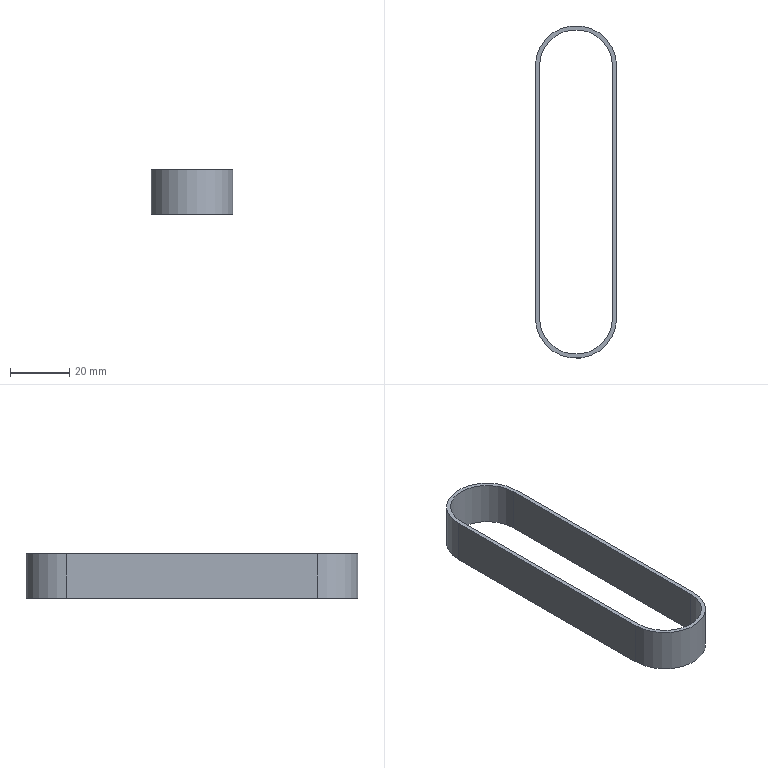Part | NX | features BREP 1 | 1 solid | 10 faces | box 27.59 x 112.59 x 15 mm | volume 5223 mm3 | plane 6 | cylinder 4 | commonest cylinder face diameters 24.83 x2 27.59 x2
STEP:
#1=CARTESIAN_POINT('',(-12.415,42.5,0.));
#2=VERTEX_POINT('',#1);
#3=CARTESIAN_POINT('',(-12.415,-42.5,0.));
#4=VERTEX_POINT('',#3);
#5=CARTESIAN_POINT('',(-12.415,-42.5,0.));
#6=DIRECTION('',(0.,-1.,0.));
#7=VECTOR('',#6,1000.);
#8=LINE('',#5,#7);
#9=EDGE_CURVE('',#2,#4,#8,.T.);
#10=ORIENTED_EDGE('',*,*,#9,.F.);
#11=CARTESIAN_POINT('',(-12.415,42.5,15.));
#12=VERTEX_POINT('',#11);
#13=CARTESIAN_POINT('',(-12.415,42.5,15.));
#14=DIRECTION('',(0.,0.,-1.));
#15=VECTOR('',#14,1000.);
#16=LINE('',#13,#15);
#17=EDGE_CURVE('',#12,#2,#16,.T.);
#18=ORIENTED_EDGE('',*,*,#17,.F.);
#19=CARTESIAN_POINT('',(-12.415,-42.5,15.));
#20=VERTEX_POINT('',#19);
#21=CARTESIAN_POINT('',(-12.415,-42.5,15.));
#22=DIRECTION('',(0.,-1.,0.));
#23=VECTOR('',#22,1000.);
#24=LINE('',#21,#23);
#25=EDGE_CURVE('',#12,#20,#24,.T.);
#26=ORIENTED_EDGE('',*,*,#25,.T.);
#27=CARTESIAN_POINT('',(-12.415,-42.5,15.));
#28=DIRECTION('',(0.,0.,-1.));
#29=VECTOR('',#28,1000.);
#30=LINE('',#27,#29);
#31=EDGE_CURVE('',#20,#4,#30,.T.);
#32=ORIENTED_EDGE('',*,*,#31,.T.);
#33=EDGE_LOOP('',(#10,#18,#26,#32));
#34=FACE_BOUND('',#33,.T.);
#35=CARTESIAN_POINT('',(-12.415,-42.5,15.));
#36=DIRECTION('',(1.,0.,0.));
#37=DIRECTION('',(0.,1.,0.));
#38=AXIS2_PLACEMENT_3D('',#35,#36,#37);
#39=PLANE('',#38);
#40=ADVANCED_FACE('',(#34),#39,.T.);
#41=CARTESIAN_POINT('',(12.415,42.5,0.));
#42=VERTEX_POINT('',#41);
#43=CARTESIAN_POINT('',(0.,42.5,0.));
#44=DIRECTION('',(0.,0.,1.));
#45=DIRECTION('',(1.,0.,0.));
#46=AXIS2_PLACEMENT_3D('',#43,#44,#45);
#47=CIRCLE('',#46,12.415);
#48=EDGE_CURVE('',#42,#2,#47,.T.);
#49=ORIENTED_EDGE('',*,*,#48,.F.);
#50=CARTESIAN_POINT('',(12.415,42.5,15.));
#51=VERTEX_POINT('',#50);
#52=CARTESIAN_POINT('',(12.415,42.5,15.));
#53=DIRECTION('',(0.,0.,-1.));
#54=VECTOR('',#53,1000.);
#55=LINE('',#52,#54);
#56=EDGE_CURVE('',#51,#42,#55,.T.);
#57=ORIENTED_EDGE('',*,*,#56,.F.);
#58=CARTESIAN_POINT('',(0.,42.5,15.));
#59=DIRECTION('',(0.,0.,1.));
#60=DIRECTION('',(1.,0.,0.));
#61=AXIS2_PLACEMENT_3D('',#58,#59,#60);
#62=CIRCLE('',#61,12.415);
#63=EDGE_CURVE('',#51,#12,#62,.T.);
#64=ORIENTED_EDGE('',*,*,#63,.T.);
#65=ORIENTED_EDGE('',*,*,#17,.T.);
#66=EDGE_LOOP('',(#49,#57,#64,#65));
#67=FACE_BOUND('',#66,.T.);
#68=CARTESIAN_POINT('',(0.,42.5,15.));
#69=DIRECTION('',(0.,0.,-1.));
#70=DIRECTION('',(-1.,0.,0.));
#71=AXIS2_PLACEMENT_3D('',#68,#69,#70);
#72=CYLINDRICAL_SURFACE('',#71,12.415);
#73=ADVANCED_FACE('',(#67),#72,.F.);
#74=CARTESIAN_POINT('',(12.415,-42.5,0.));
#75=VERTEX_POINT('',#74);
#76=CARTESIAN_POINT('',(12.415,-42.5,0.));
#77=DIRECTION('',(0.,1.,0.));
#78=VECTOR('',#77,1000.);
#79=LINE('',#76,#78);
#80=EDGE_CURVE('',#75,#42,#79,.T.);
#81=ORIENTED_EDGE('',*,*,#80,.F.);
#82=CARTESIAN_POINT('',(12.415,-42.5,15.));
#83=VERTEX_POINT('',#82);
#84=CARTESIAN_POINT('',(12.415,-42.5,15.));
#85=DIRECTION('',(0.,0.,-1.));
#86=VECTOR('',#85,1000.);
#87=LINE('',#84,#86);
#88=EDGE_CURVE('',#83,#75,#87,.T.);
#89=ORIENTED_EDGE('',*,*,#88,.F.);
#90=CARTESIAN_POINT('',(12.415,-42.5,15.));
#91=DIRECTION('',(0.,1.,0.));
#92=VECTOR('',#91,1000.);
#93=LINE('',#90,#92);
#94=EDGE_CURVE('',#83,#51,#93,.T.);
#95=ORIENTED_EDGE('',*,*,#94,.T.);
#96=ORIENTED_EDGE('',*,*,#56,.T.);
#97=EDGE_LOOP('',(#81,#89,#95,#96));
#98=FACE_BOUND('',#97,.T.);
#99=CARTESIAN_POINT('',(12.415,-42.5,15.));
#100=DIRECTION('',(-1.,0.,0.));
#101=DIRECTION('',(0.,-1.,0.));
#102=AXIS2_PLACEMENT_3D('',#99,#100,#101);
#103=PLANE('',#102);
#104=ADVANCED_FACE('',(#98),#103,.T.);
#105=CARTESIAN_POINT('',(0.,-42.5,0.));
#106=DIRECTION('',(0.,0.,1.));
#107=DIRECTION('',(1.,0.,0.));
#108=AXIS2_PLACEMENT_3D('',#105,#106,#107);
#109=CIRCLE('',#108,12.415);
#110=EDGE_CURVE('',#4,#75,#109,.T.);
#111=ORIENTED_EDGE('',*,*,#110,.F.);
#112=ORIENTED_EDGE('',*,*,#31,.F.);
#113=CARTESIAN_POINT('',(0.,-42.5,15.));
#114=DIRECTION('',(0.,0.,1.));
#115=DIRECTION('',(1.,0.,0.));
#116=AXIS2_PLACEMENT_3D('',#113,#114,#115);
#117=CIRCLE('',#116,12.415);
#118=EDGE_CURVE('',#20,#83,#117,.T.);
#119=ORIENTED_EDGE('',*,*,#118,.T.);
#120=ORIENTED_EDGE('',*,*,#88,.T.);
#121=EDGE_LOOP('',(#111,#112,#119,#120));
#122=FACE_BOUND('',#121,.T.);
#123=CARTESIAN_POINT('',(0.,-42.5,15.));
#124=DIRECTION('',(0.,0.,-1.));
#125=DIRECTION('',(-1.,0.,0.));
#126=AXIS2_PLACEMENT_3D('',#123,#124,#125);
#127=CYLINDRICAL_SURFACE('',#126,12.415);
#128=ADVANCED_FACE('',(#122),#127,.F.);
#129=CARTESIAN_POINT('',(-13.795,42.5,0.));
#130=VERTEX_POINT('',#129);
#131=CARTESIAN_POINT('',(-13.795,-42.5,0.));
#132=VERTEX_POINT('',#131);
#133=CARTESIAN_POINT('',(-13.795,-42.5,0.));
#134=DIRECTION('',(0.,-1.,0.));
#135=VECTOR('',#134,1000.);
#136=LINE('',#133,#135);
#137=EDGE_CURVE('',#130,#132,#136,.T.);
#138=ORIENTED_EDGE('',*,*,#137,.T.);
#139=CARTESIAN_POINT('',(-13.795,-42.5,15.));
#140=VERTEX_POINT('',#139);
#141=CARTESIAN_POINT('',(-13.795,-42.5,15.));
#142=DIRECTION('',(0.,0.,-1.));
#143=VECTOR('',#142,1000.);
#144=LINE('',#141,#143);
#145=EDGE_CURVE('',#140,#132,#144,.T.);
#146=ORIENTED_EDGE('',*,*,#145,.F.);
#147=CARTESIAN_POINT('',(-13.795,42.5,15.));
#148=VERTEX_POINT('',#147);
#149=CARTESIAN_POINT('',(-13.795,-42.5,15.));
#150=DIRECTION('',(0.,-1.,0.));
#151=VECTOR('',#150,1000.);
#152=LINE('',#149,#151);
#153=EDGE_CURVE('',#148,#140,#152,.T.);
#154=ORIENTED_EDGE('',*,*,#153,.F.);
#155=CARTESIAN_POINT('',(-13.795,42.5,15.));
#156=DIRECTION('',(0.,0.,-1.));
#157=VECTOR('',#156,1000.);
#158=LINE('',#155,#157);
#159=EDGE_CURVE('',#148,#130,#158,.T.);
#160=ORIENTED_EDGE('',*,*,#159,.T.);
#161=EDGE_LOOP('',(#138,#146,#154,#160));
#162=FACE_BOUND('',#161,.T.);
#163=CARTESIAN_POINT('',(-13.795,-42.5,15.));
#164=DIRECTION('',(1.,0.,0.));
#165=DIRECTION('',(0.,1.,0.));
#166=AXIS2_PLACEMENT_3D('',#163,#164,#165);
#167=PLANE('',#166);
#168=ADVANCED_FACE('',(#162),#167,.F.);
#169=CARTESIAN_POINT('',(13.795,42.5,0.));
#170=VERTEX_POINT('',#169);
#171=CARTESIAN_POINT('',(0.,42.5,0.));
#172=DIRECTION('',(0.,0.,1.));
#173=DIRECTION('',(1.,0.,0.));
#174=AXIS2_PLACEMENT_3D('',#171,#172,#173);
#175=CIRCLE('',#174,13.795);
#176=EDGE_CURVE('',#170,#130,#175,.T.);
#177=ORIENTED_EDGE('',*,*,#176,.T.);
#178=ORIENTED_EDGE('',*,*,#159,.F.);
#179=CARTESIAN_POINT('',(13.795,42.5,15.));
#180=VERTEX_POINT('',#179);
#181=CARTESIAN_POINT('',(0.,42.5,15.));
#182=DIRECTION('',(0.,0.,1.));
#183=DIRECTION('',(1.,0.,0.));
#184=AXIS2_PLACEMENT_3D('',#181,#182,#183);
#185=CIRCLE('',#184,13.795);
#186=EDGE_CURVE('',#180,#148,#185,.T.);
#187=ORIENTED_EDGE('',*,*,#186,.F.);
#188=CARTESIAN_POINT('',(13.795,42.5,15.));
#189=DIRECTION('',(0.,0.,-1.));
#190=VECTOR('',#189,1000.);
#191=LINE('',#188,#190);
#192=EDGE_CURVE('',#180,#170,#191,.T.);
#193=ORIENTED_EDGE('',*,*,#192,.T.);
#194=EDGE_LOOP('',(#177,#178,#187,#193));
#195=FACE_BOUND('',#194,.T.);
#196=CARTESIAN_POINT('',(0.,42.5,15.));
#197=DIRECTION('',(0.,0.,-1.));
#198=DIRECTION('',(-1.,0.,0.));
#199=AXIS2_PLACEMENT_3D('',#196,#197,#198);
#200=CYLINDRICAL_SURFACE('',#199,13.795);
#201=ADVANCED_FACE('',(#195),#200,.T.);
#202=CARTESIAN_POINT('',(13.795,-42.5,0.));
#203=VERTEX_POINT('',#202);
#204=CARTESIAN_POINT('',(13.795,-42.5,0.));
#205=DIRECTION('',(0.,1.,0.));
#206=VECTOR('',#205,1000.);
#207=LINE('',#204,#206);
#208=EDGE_CURVE('',#203,#170,#207,.T.);
#209=ORIENTED_EDGE('',*,*,#208,.T.);
#210=ORIENTED_EDGE('',*,*,#192,.F.);
#211=CARTESIAN_POINT('',(13.795,-42.5,15.));
#212=VERTEX_POINT('',#211);
#213=CARTESIAN_POINT('',(13.795,-42.5,15.));
#214=DIRECTION('',(0.,1.,0.));
#215=VECTOR('',#214,1000.);
#216=LINE('',#213,#215);
#217=EDGE_CURVE('',#212,#180,#216,.T.);
#218=ORIENTED_EDGE('',*,*,#217,.F.);
#219=CARTESIAN_POINT('',(13.795,-42.5,15.));
#220=DIRECTION('',(0.,0.,-1.));
#221=VECTOR('',#220,1000.);
#222=LINE('',#219,#221);
#223=EDGE_CURVE('',#212,#203,#222,.T.);
#224=ORIENTED_EDGE('',*,*,#223,.T.);
#225=EDGE_LOOP('',(#209,#210,#218,#224));
#226=FACE_BOUND('',#225,.T.);
#227=CARTESIAN_POINT('',(13.795,-42.5,15.));
#228=DIRECTION('',(-1.,0.,0.));
#229=DIRECTION('',(0.,-1.,0.));
#230=AXIS2_PLACEMENT_3D('',#227,#228,#229);
#231=PLANE('',#230);
#232=ADVANCED_FACE('',(#226),#231,.F.);
#233=CARTESIAN_POINT('',(0.,-42.5,0.));
#234=DIRECTION('',(0.,0.,1.));
#235=DIRECTION('',(1.,0.,0.));
#236=AXIS2_PLACEMENT_3D('',#233,#234,#235);
#237=CIRCLE('',#236,13.795);
#238=EDGE_CURVE('',#132,#203,#237,.T.);
#239=ORIENTED_EDGE('',*,*,#238,.T.);
#240=ORIENTED_EDGE('',*,*,#223,.F.);
#241=CARTESIAN_POINT('',(0.,-42.5,15.));
#242=DIRECTION('',(0.,0.,1.));
#243=DIRECTION('',(1.,0.,0.));
#244=AXIS2_PLACEMENT_3D('',#241,#242,#243);
#245=CIRCLE('',#244,13.795);
#246=EDGE_CURVE('',#140,#212,#245,.T.);
#247=ORIENTED_EDGE('',*,*,#246,.F.);
#248=ORIENTED_EDGE('',*,*,#145,.T.);
#249=EDGE_LOOP('',(#239,#240,#247,#248));
#250=FACE_BOUND('',#249,.T.);
#251=CARTESIAN_POINT('',(0.,-42.5,15.));
#252=DIRECTION('',(0.,0.,-1.));
#253=DIRECTION('',(-1.,0.,0.));
#254=AXIS2_PLACEMENT_3D('',#251,#252,#253);
#255=CYLINDRICAL_SURFACE('',#254,13.795);
#256=ADVANCED_FACE('',(#250),#255,.T.);
#257=ORIENTED_EDGE('',*,*,#110,.T.);
#258=ORIENTED_EDGE('',*,*,#80,.T.);
#259=ORIENTED_EDGE('',*,*,#48,.T.);
#260=ORIENTED_EDGE('',*,*,#9,.T.);
#261=EDGE_LOOP('',(#257,#258,#259,#260));
#262=FACE_BOUND('',#261,.T.);
#263=ORIENTED_EDGE('',*,*,#238,.F.);
#264=ORIENTED_EDGE('',*,*,#137,.F.);
#265=ORIENTED_EDGE('',*,*,#176,.F.);
#266=ORIENTED_EDGE('',*,*,#208,.F.);
#267=EDGE_LOOP('',(#263,#264,#265,#266));
#268=FACE_BOUND('',#267,.T.);
#269=CARTESIAN_POINT('',(0.,-42.5,0.));
#270=DIRECTION('',(0.,0.,1.));
#271=DIRECTION('',(1.,0.,0.));
#272=AXIS2_PLACEMENT_3D('',#269,#270,#271);
#273=PLANE('',#272);
#274=ADVANCED_FACE('',(#262,#268),#273,.F.);
#275=ORIENTED_EDGE('',*,*,#94,.F.);
#276=ORIENTED_EDGE('',*,*,#118,.F.);
#277=ORIENTED_EDGE('',*,*,#25,.F.);
#278=ORIENTED_EDGE('',*,*,#63,.F.);
#279=EDGE_LOOP('',(#275,#276,#277,#278));
#280=FACE_BOUND('',#279,.T.);
#281=ORIENTED_EDGE('',*,*,#246,.T.);
#282=ORIENTED_EDGE('',*,*,#217,.T.);
#283=ORIENTED_EDGE('',*,*,#186,.T.);
#284=ORIENTED_EDGE('',*,*,#153,.T.);
#285=EDGE_LOOP('',(#281,#282,#283,#284));
#286=FACE_BOUND('',#285,.T.);
#287=CARTESIAN_POINT('',(0.,-42.5,15.));
#288=DIRECTION('',(0.,0.,1.));
#289=DIRECTION('',(1.,0.,0.));
#290=AXIS2_PLACEMENT_3D('',#287,#288,#289);
#291=PLANE('',#290);
#292=ADVANCED_FACE('',(#280,#286),#291,.T.);
#293=CLOSED_SHELL('',(#40,#73,#104,#128,#168,#201,#232,#256,#274,#292));
#294=MANIFOLD_SOLID_BREP('',#293);
#295=(LENGTH_UNIT()NAMED_UNIT(*)SI_UNIT(.MILLI.,.METRE.));
#296=UNCERTAINTY_MEASURE_WITH_UNIT(LENGTH_MEASURE(0.00001),#295,'','');
#297=(NAMED_UNIT(*)PLANE_ANGLE_UNIT()SI_UNIT($,.RADIAN.));
#298=(NAMED_UNIT(*)SI_UNIT($,.STERADIAN.)SOLID_ANGLE_UNIT());
#299=(GEOMETRIC_REPRESENTATION_CONTEXT(3)GLOBAL_UNCERTAINTY_ASSIGNED_CONTEXT((#296))GLOBAL_UNIT_ASSIGNED_CONTEXT((#295,#297,#298))REPRESENTATION_CONTEXT('',''));
#300=ADVANCED_BREP_SHAPE_REPRESENTATION('',(#294),#299);